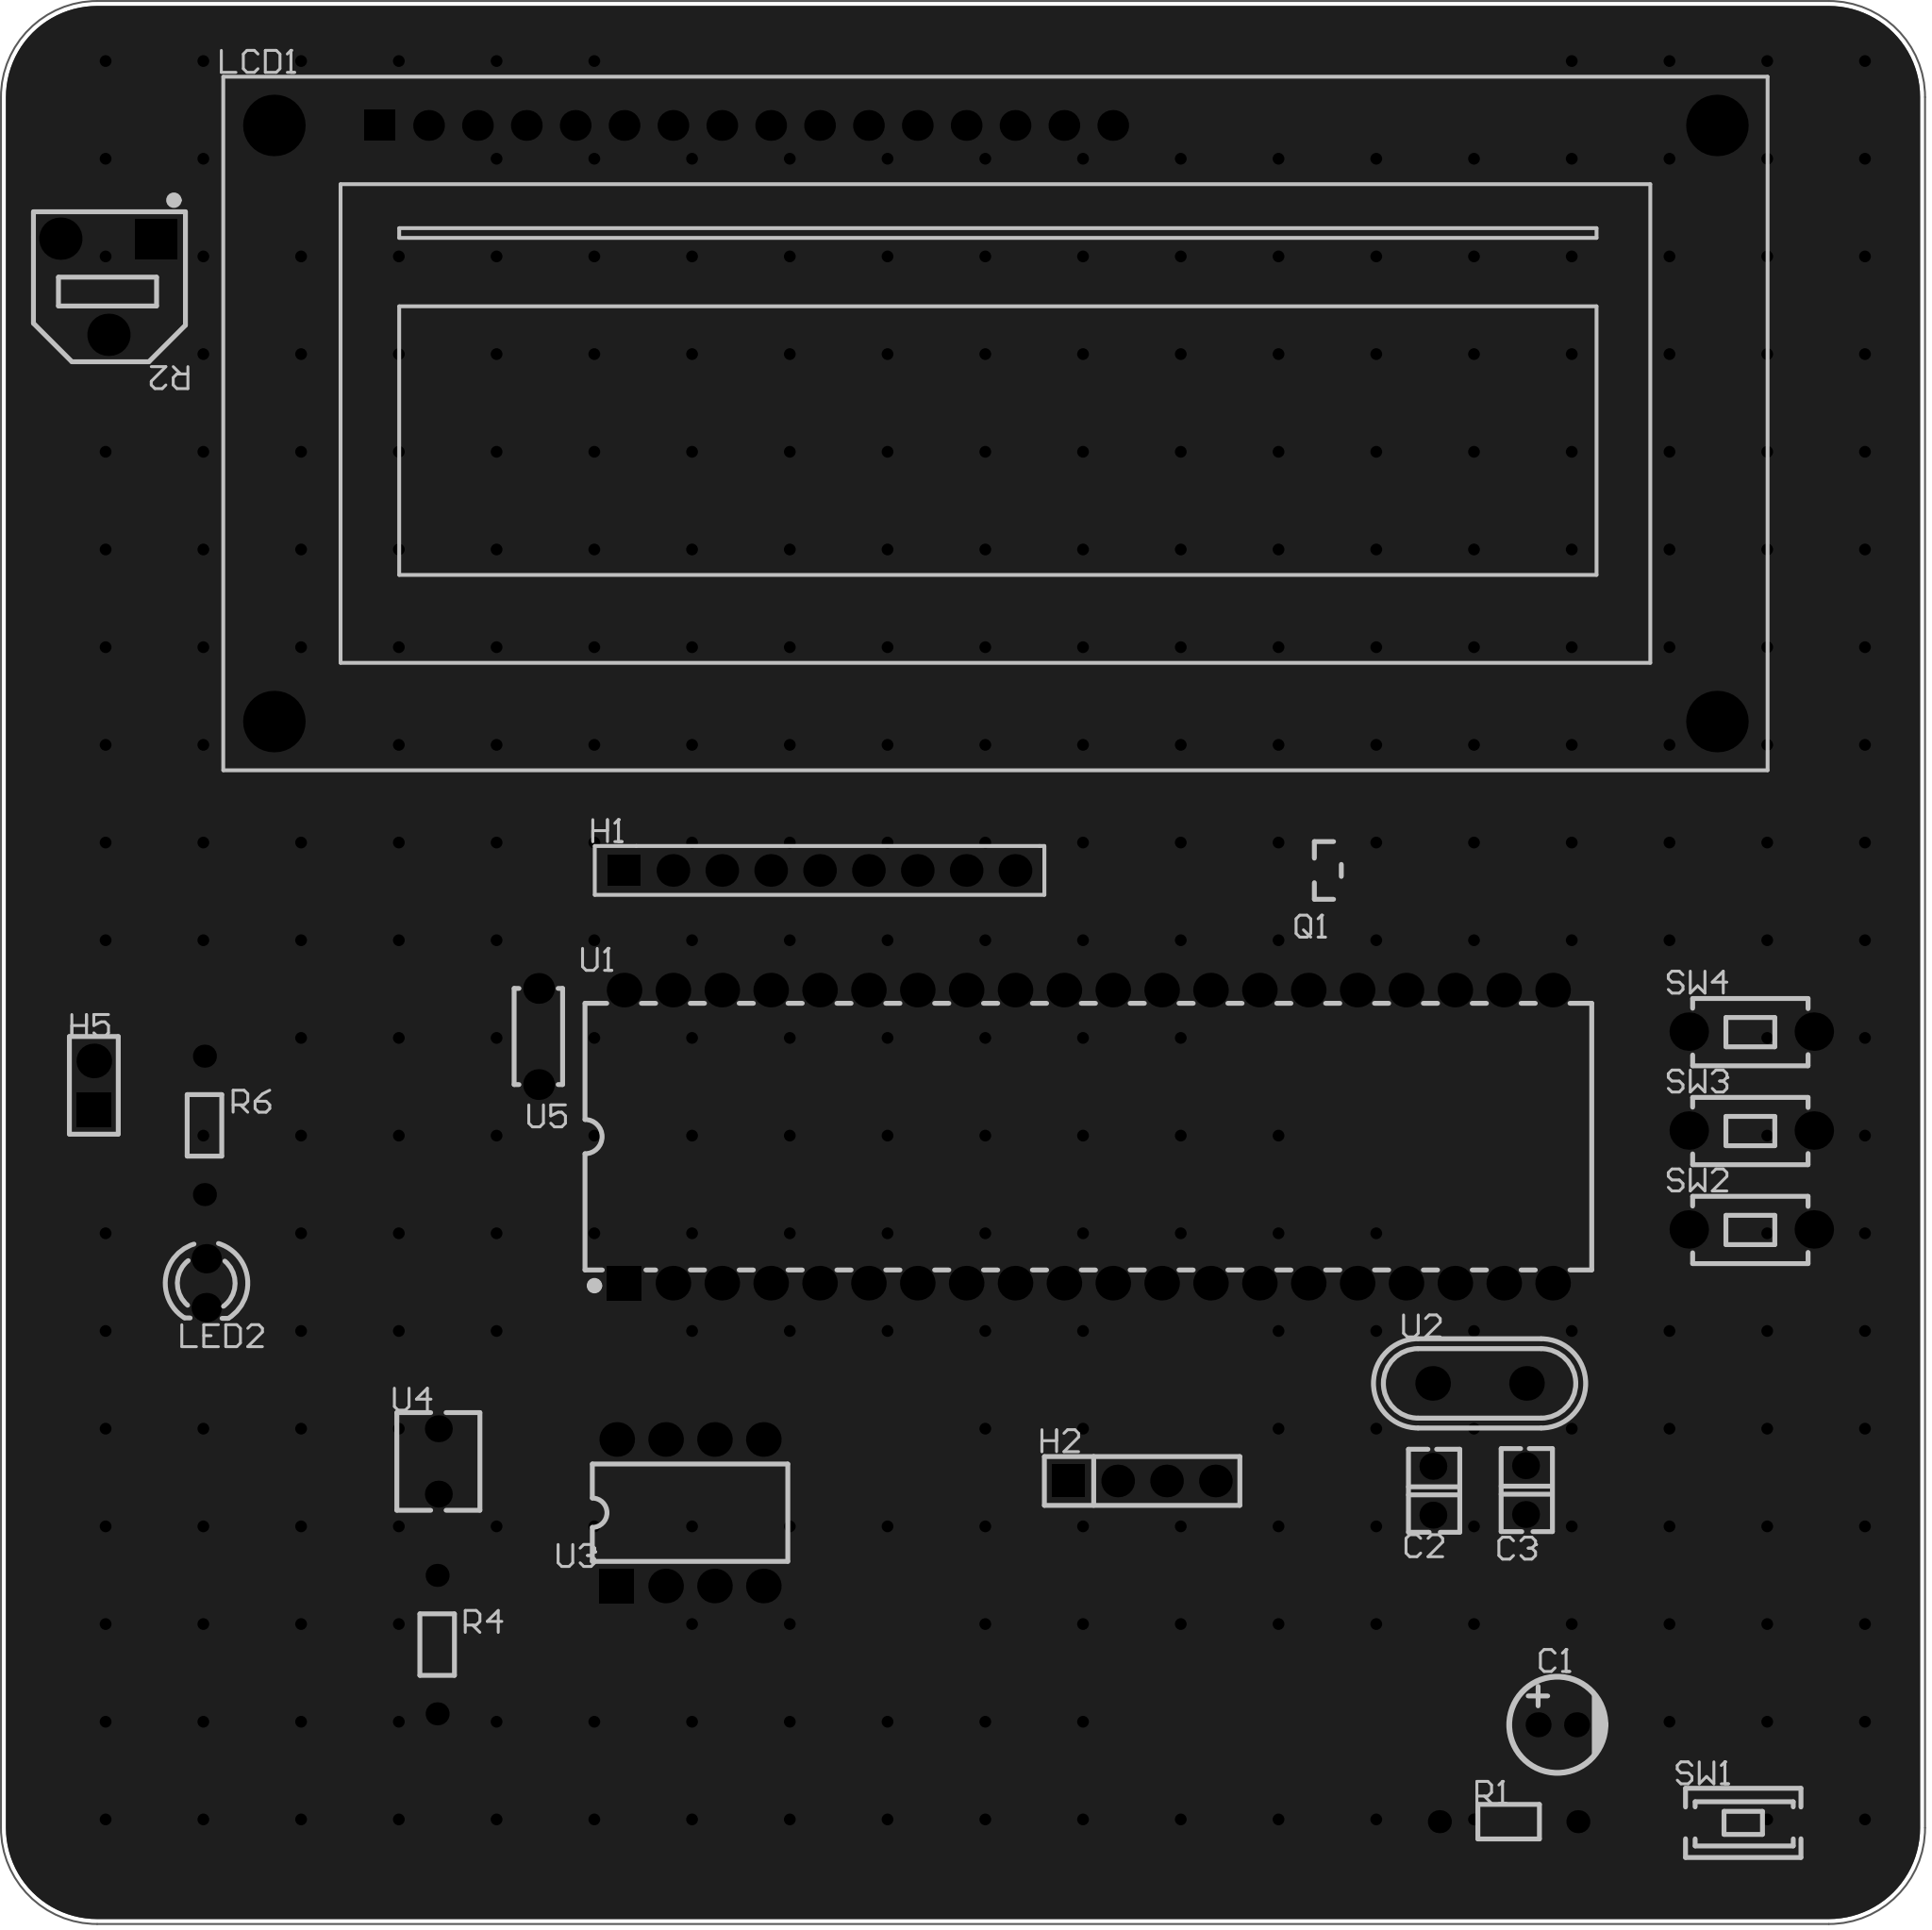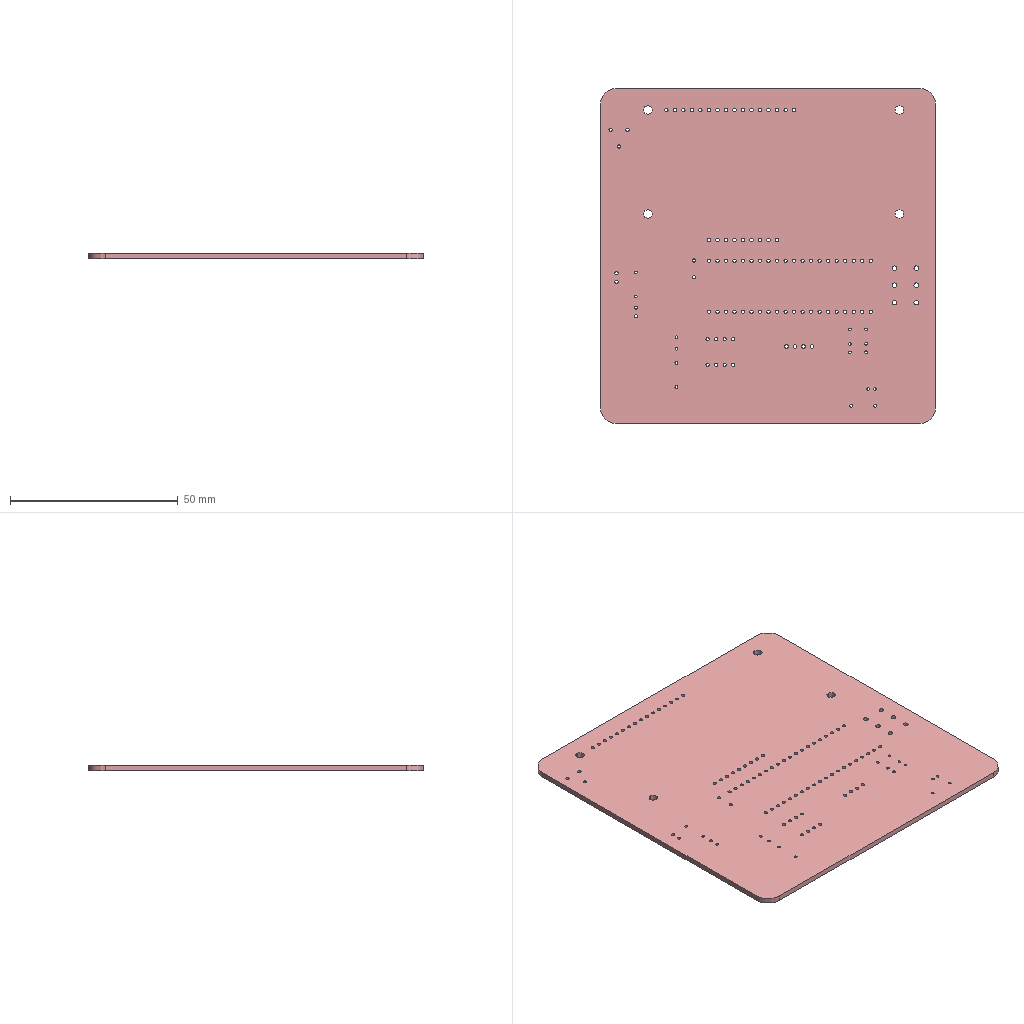Circuit board layout | Altium Designer | box 100 x 100 x 1.6 mm
Layer stack:
# Altium Designer layer stack of  (unit mm; dielectric type: 0 none, 1 core, 2 prepreg, 3 surface material)
index,name,kind,layer,copper_thickness_mm,dielectric_type,dielectric_thickness_mm,dielectric_material,dielectric_constant
0,Top Paste Mask Layer,other,,,,,,
1,Top Silkscreen Layer,other,,,,,,
2,Top Solder Mask Layer,dielectric,,,3,0.01,,3.3
3,Top Layer,copper,Top Layer,0.035,,,,
4,Dielectric1,dielectric,,,3,1.51,FR4,4.5
5,Bottom Layer,copper,Bottom Layer,0.035,,,,
6,Bottom Solder Mask Layer,dielectric,,,3,0.01,,3.3
7,Bottom Silkscreen Layer,other,,,,,,
8,Bottom Paste Mask Layer,other,,,,,,
# drill layer pairs: low layer,high layer
drill_pair,Top Layer,Bottom Layer
Part placement:
Designator,Comment,Layer,Footprint,Center-X(mm),Center-Y(mm),Rotation
H1,,TopLayer,HDR-TH_9P-P2.54-V-F-1,125.222,142.367,0
LCD1,LMB162ADC,TopLayer,LCD1602,134.362,165.608,0
U1,STC89C516RD+40I-PDIP40,TopLayer,DIP-40_L52.3-W13.9-P2.54-LS15.2-BL,139.192,128.524,0
U2,11.059MHz,TopLayer,HC-49US_L11.0-W4.6-P4.88,159.525,115.692,0
H5,,TopLayer,HDR-TH_2P-P2.54-V-M-1,87.503,131.191,90
SW1,Tact switch 3*6*2.5,TopLayer,SW-SMD_L6.0-W3.6-LS8.0,173.228,92.837,0
R4,10kΩ,TopLayer,Res_1/8W,105.347,102.108,90
U3,ADC0832CCN,TopLayer,DIP-8_L9.7-W6.4-P2.54-LS7.6-BL,118.491,108.966,0
U4,光敏电阻-5MM,TopLayer,RES-TH_L4.9-W4.3-P3.4,105.41,111.633,270
C1,10uF,TopLayer,CAP-TH_BD5.0-P2.00-D0.8-FD-10UF50VC110GL,163.566,97.938,0
C2,30pF,TopLayer,CAP-TH_L3.8-W2.5-P2.54-D0.50,157.099,110.109,90
C3,30pF,TopLayer,CAP-TH_L3.8-W2.5-P2.54-D0.50,161.915,110.143,90
R1,10kΩ,TopLayer,Res_1/8W,161.036,92.9,0
LED2,,TopLayer,LED_TH-3mm,93.345,120.904,270
R6,220Ω,TopLayer,Res_1/8W,93.253,129.109,90
H2,,TopLayer,HDR-TH_4P-P2.54-V-M,141.986,110.617,0
Q1,,TopLayer,S8050_SOT-23,151.638,142.367,0
R2,10kΩ,TopLayer,RES-ADJ-SMD_RM065-V1,88.265,172.72,180
SW2,,TopLayer,Key_TH_3.5x6x4.3,173.647,123.698,0
SW3,,TopLayer,Key_TH_3.5x6x4.3,173.647,128.841,0
SW4,,TopLayer,Key_TH_3.5x6x4.3,173.647,133.985,0
U5,100nF,TopLayer,CAP-TH_L5.0-W2.5-P5.00-D1.0,110.617,133.731,270
Pad and via stacks:
# Altium Designer via and pad stacks of  (unit mm). Each distinct definition once, with the count of objects using it.
# via: kind,start_layer,end_layer,hole_mm,diameter_mm,mode(0 simple;1 top-mid-bottom;2 full stack),diameter_per_layer,count,example_net
# pad: kind,layer,hole_mm,hole_type(0 round;1 square;2 slot),plating,top_size,top_shape(1 round;2 rect;3 octagon;9 rounded rect),mid_size,bottom_size,mode,footprint,size_per_layer,count,example
pad,Multi-Layer,1.1,0,plated,1.7x1.575,2,1.7x1.575,1.7x1.575,0,HDR-TH_9P-P2.54-V-F-1,,1,H1.1
pad,Multi-Layer,1.1,0,plated,1.7x1.7,1,1.7x1.7,1.7x1.7,0,HDR-TH_9P-P2.54-V-F-1,,8,H1.2
pad,Multi-Layer,1,0,plated,1.6x1.6,1,1.6x1.6,1.6x1.6,0,LCD1602,,15,LCD1.16
pad,Multi-Layer,1,0,plated,1.6x1.6,2,1.6x1.6,1.6x1.6,0,LCD1602,,1,LCD1.1
pad,Multi-Layer,2.5,2,plated,3.2x3.2,1,3.2x3.2,3.2x3.2,0,LCD1602,,4,LCD1.0
pad,Multi-Layer,1,0,plated,1.8x1.8,1,1.8x1.8,1.8x1.8,0,DIP-40_L52.3-W13.9-P2.54-LS15.2-BL,,39,U1.19
pad,Multi-Layer,1,0,plated,1.8x1.8,2,1.8x1.8,1.8x1.8,0,DIP-40_L52.3-W13.9-P2.54-LS15.2-BL,,1,U1.1
pad,Multi-Layer,0.8,0,plated,1.8x1.8,1,1.8x1.8,1.8x1.8,0,HC-49US_L11.0-W4.6-P4.88,,2,U2.1
pad,Multi-Layer,1,0,plated,1.8x1.8,1,1.8x1.8,1.8x1.8,0,HDR-TH_2P-P2.54-V-M-1,,1,H5.2
pad,Multi-Layer,1,0,plated,1.8x1.8,2,1.8x1.8,1.8x1.8,0,HDR-TH_2P-P2.54-V-M-1,,1,H5.1
pad,Multi-Layer,0.8001,0,plated,1.199x1.199,1,1.199x1.199,1.199x1.199,0,Res_1/8W,,6,R4.1
pad,Multi-Layer,1,0,plated,1.8x1.8,2,1.8x1.8,1.8x1.8,0,DIP-8_L9.7-W6.4-P2.54-LS7.6-BL,,1,U3.1
pad,Multi-Layer,1,0,plated,1.8x1.8,1,1.8x1.8,1.8x1.8,0,DIP-8_L9.7-W6.4-P2.54-LS7.6-BL,,7,U3.2
pad,Multi-Layer,0.8,0,plated,1.4x1.4,1,1.4x1.4,1.4x1.4,0,RES-TH_L4.9-W4.3-P3.4,,2,U4.1
pad,Multi-Layer,0.8,0,plated,1.3x1.3,1,1.3x1.3,1.3x1.3,0,CAP-TH_BD5.0-P2.00-D0.8-FD-10UF50VC110GL,,2,C1.2
pad,Multi-Layer,0.8,0,plated,1.4x1.4,1,1.4x1.4,1.4x1.4,0,CAP-TH_L3.8-W2.5-P2.54-D0.50,,4,C2.1
pad,Multi-Layer,0.9144,0,plated,1.524x1.524,1,1.524x1.524,1.524x1.524,0,LED_TH-3mm,,2,LED2.1
pad,Multi-Layer,1.1,0,plated,1.7x1.7,2,1.7x1.7,1.7x1.7,0,HDR-TH_4P-P2.54-V-M,,1,H2.1
pad,Multi-Layer,1.1,0,plated,1.7x1.7,1,1.7x1.7,1.7x1.7,0,HDR-TH_4P-P2.54-V-M,,3,H2.2
pad,Multi-Layer,1,0,plated,2.2x2.1,2,2.2x2.1,2.2x2.1,0,RES-ADJ-SMD_RM065-V1,,1,R2.1
pad,Multi-Layer,1,0,plated,2.2x2.2,1,2.2x2.2,2.2x2.2,0,RES-ADJ-SMD_RM065-V1,,2,R2.3
pad,Multi-Layer,1.399,0,plated,1.999x1.999,1,1.999x1.999,1.999x1.999,0,Key_TH_3.5x6x4.3,,6,SW2.A
pad,Multi-Layer,1,0,plated,1.6x1.6,1,1.6x1.6,1.6x1.6,0,CAP-TH_L5.0-W2.5-P5.00-D1.0,,2,U5.1
pad,Top Layer,0,0,plated,1.5x1,2,1.5x1,1.5x1,0,SW-SMD_L6.0-W3.6-LS8.0,,2,SW1.1
pad,Top Layer,0,0,plated,1x0.8,2,1x0.8,1x0.8,0,S8050_SOT-23,,3,Q1.2
via,Top Layer,Bottom Layer,0.3048,0.61,0,,313,GND
Copper pours:
name,layer,net,type(0 solid;1 hatched;2 none)
Top Layer-GND,Top Layer,GND,0
Bottom Layer-GND,Bottom Layer,GND,0